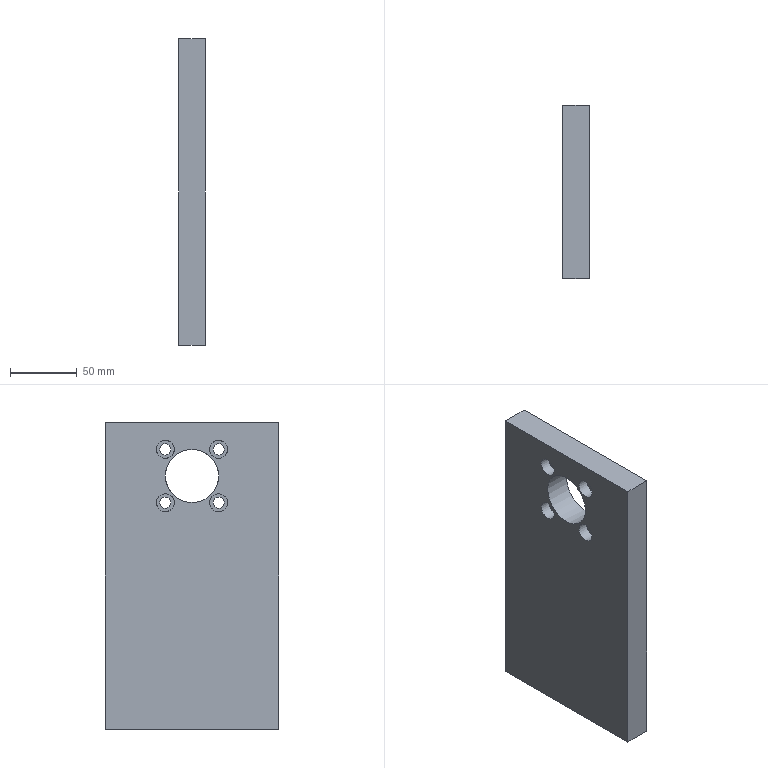Part | STEP file | Tube necking machine_id550_x_t | 1 solid | 19 faces | box 20 x 130 x 230 mm | volume 565563 mm3 | plane 10 | cylinder 9 | commonest cylinder face diameters 8.5 x4 13.5 x4 40 x1